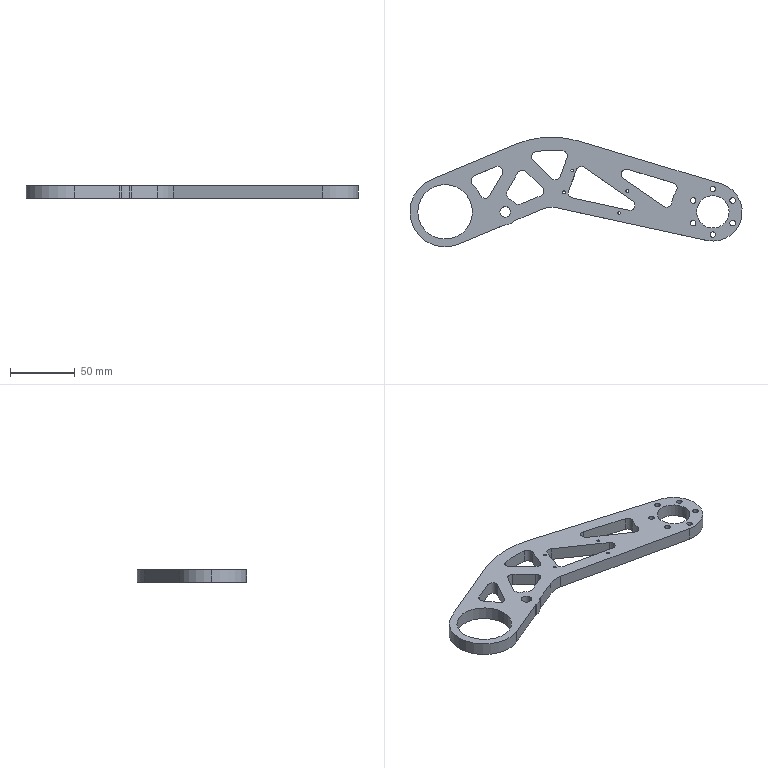Part | SolidWorks | features ICE 7, Fillet 2, Extrusion 1 | 1 solid | 79 faces | box 255.5 x 84.429 x 10 mm | volume 83626 mm3 | cylinder 60 | plane 19 | commonest cylinder face diameters 8 x21 4.2 x12 2.2 x8 10 x4 20 x2 25 x2